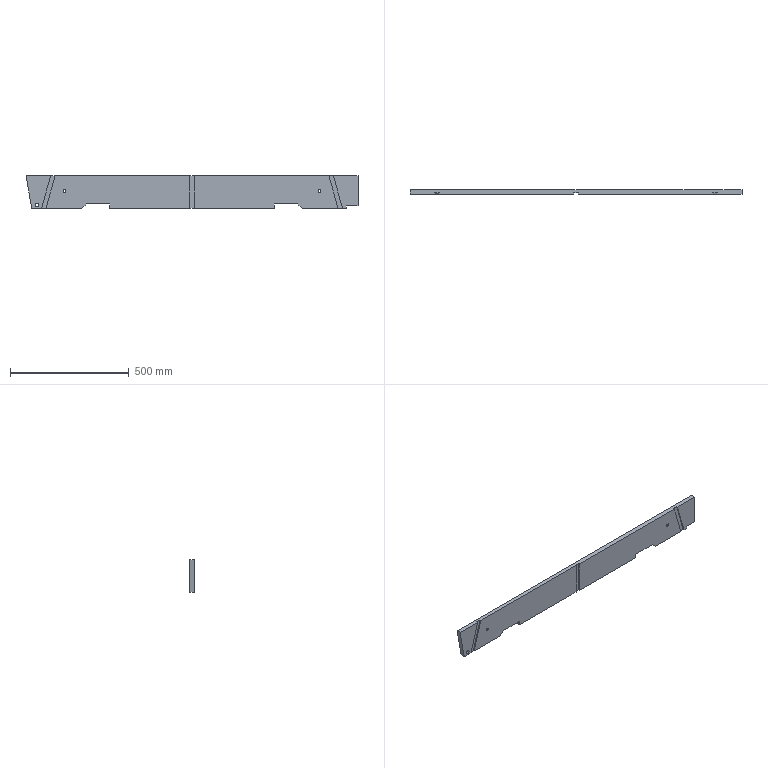Part | STEP file | Frame_right | 1 solid | 31 faces | box 1400 x 18 x 137 mm | volume 3298397 mm3 | plane 28 | cylinder 3 | commonest cylinder face diameters 11 x2 15 x1